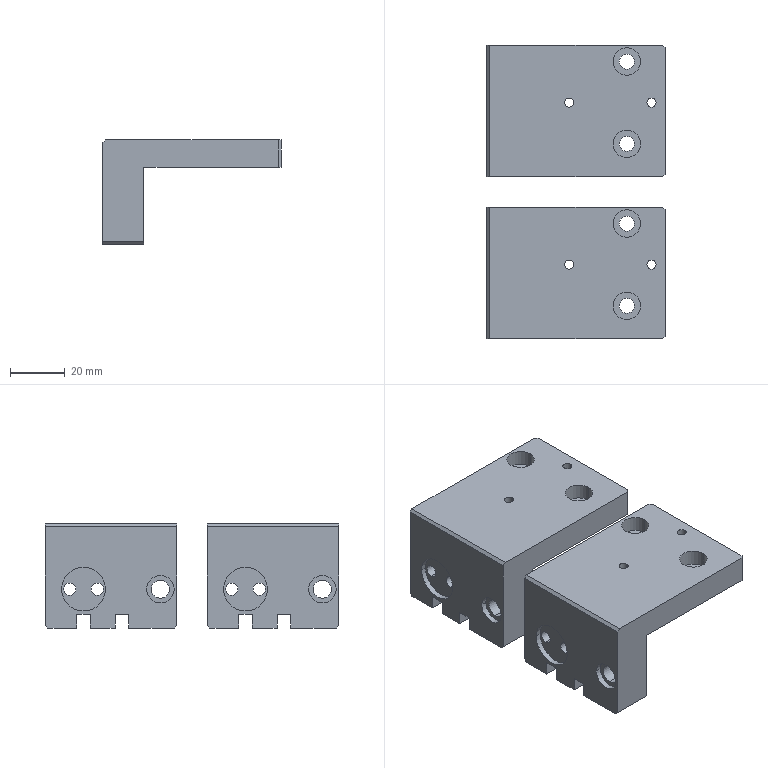NC program | NX | posted with a generic post | part box 65 x 107 x 38 mm
Lines 5400 to 5955 of 5955:
(ZLEVEL_PROFILE_COPY_1 , TOOL : D10JING)
N10774 T14 M6
N10776 G54
N10778 G17 G0 G90 X0.5 Y-6.567 B0. C0. S9500 M3
N10780 G43 Z30. H14
N10782 Z1.5
N10784 G94 G1 Y33.049 Z-0.576 F1000.
N10786 X0.828 Y34.364 Z-0.647
N10788 X1.496 Y35.545 Z-0.718
N10790 X2.455 Y36.504 Z-0.789
N10792 X3.636 Y37.172 Z-0.86
N10794 X4.951 Y37.5 Z-0.932
N10796 X54.049 Z-3.505
N10798 X55.364 Y37.172 Z-3.576
N10800 X56.545 Y36.504 Z-3.647
N10802 X57.504 Y35.545 Z-3.718
N10804 X58.172 Y34.364 Z-3.789
N10806 X58.5 Y33.049 Z-3.86
N10808 Y-32.049 Z-7.272
N10810 X58.147 Y-33.425 Z-7.346
N10812 X57.423 Y-34.648 Z-7.421
N10814 X55.648 Y-36.423 Z-7.552
N10816 X54.425 Y-37.147 Z-7.627
N10818 X53.049 Y-37.5 Z-7.701
N10820 X5.951 Z-10.169
N10822 X4.575 Y-37.147 Z-10.244
N10824 X3.352 Y-36.423 Z-10.318
N10826 X1.577 Y-34.648 Z-10.45
N10828 X0.853 Y-33.425 Z-10.524
N10830 X0.5 Y-32.049 Z-10.599
N10832 Y33.049 Z-14.01
N10834 X0.828 Y34.364 Z-14.081
N10836 X1.496 Y35.545 Z-14.153
N10838 X2.455 Y36.504 Z-14.224
N10840 X3.636 Y37.172 Z-14.295
N10842 X4.951 Y37.5 Z-14.366
N10844 X54.049 Z-16.939
N10846 X55.364 Y37.172 Z-17.01
N10848 X56.545 Y36.504 Z-17.081
N10850 X57.504 Y35.545 Z-17.152
N10852 X58.172 Y34.364 Z-17.223
N10854 X58.5 Y33.049 Z-17.294
N10856 Y0.5 Z-19.
N10858 Y-31.5 F1200.
N10860 G2 X57.036 Y-35.036 R5.
N10862 G1 X56.036 Y-36.036
N10864 G2 X52.5 Y-37.5 R5.
N10866 G1 X6.5
N10868 G2 X2.964 Y-36.036 R5.
N10870 G1 X1.964 Y-35.036
N10872 G2 X0.5 Y-31.5 R5.
N10874 G1 Y32.5
N10876 G2 X5.5 Y37.5 R5.
N10878 G1 X53.5
N10880 G2 X58.5 Y32.5 R5.
N10882 G1 Y0.5
N10884 Y-31.5 Z-21.373
N10886 X58.476 Y-31.99 Z-21.41
N10888 X58.404 Y-32.475 Z-21.446
N10890 X58.285 Y-32.951 Z-21.482
N10892 X58.119 Y-33.413 Z-21.519
N10894 X57.91 Y-33.857 Z-21.555
N10896 X57.657 Y-34.278 Z-21.591
N10898 X57.365 Y-34.672 Z-21.628
N10900 X57.036 Y-35.036 Z-21.664
N10902 X56.036 Y-36.036 Z-21.769
N10904 X55.672 Y-36.365 Z-21.805
N10906 X55.278 Y-36.657 Z-21.842
N10908 X54.857 Y-36.91 Z-21.878
N10910 X54.413 Y-37.119 Z-21.914
N10912 X53.951 Y-37.285 Z-21.951
N10914 X53.475 Y-37.404 Z-21.987
N10916 X52.99 Y-37.476 Z-22.023
N10918 X52.5 Y-37.5 Z-22.06
N10920 X6.5 Z-25.471
N10922 X6.01 Y-37.476 Z-25.507
N10924 X5.525 Y-37.404 Z-25.544
N10926 X5.049 Y-37.285 Z-25.58
N10928 X4.587 Y-37.119 Z-25.616
N10930 X4.143 Y-36.91 Z-25.653
N10932 X3.722 Y-36.657 Z-25.689
N10934 X3.328 Y-36.365 Z-25.726
N10936 X2.964 Y-36.036 Z-25.762
N10938 X1.964 Y-35.036 Z-25.867
N10940 X1.635 Y-34.672 Z-25.903
N10942 X1.343 Y-34.278 Z-25.939
N10944 X1.09 Y-33.857 Z-25.976
N10946 X0.881 Y-33.413 Z-26.012
N10948 X0.715 Y-32.951 Z-26.048
N10950 X0.596 Y-32.475 Z-26.085
N10952 X0.524 Y-31.99 Z-26.121
N10954 X0.5 Y-31.5 Z-26.158
N10956 Y32.5 Z-30.904
N10958 X0.524 Y32.99 Z-30.94
N10960 X0.596 Y33.475 Z-30.977
N10962 X0.715 Y33.951 Z-31.013
N10964 X0.881 Y34.413 Z-31.049
N10966 X1.09 Y34.857 Z-31.086
N10968 X1.343 Y35.278 Z-31.122
N10970 X1.635 Y35.672 Z-31.158
N10972 X1.964 Y36.036 Z-31.195
N10974 X2.328 Y36.365 Z-31.231
N10976 X2.722 Y36.657 Z-31.267
N10978 X3.143 Y36.91 Z-31.304
N10980 X3.587 Y37.119 Z-31.34
N10982 X4.049 Y37.285 Z-31.376
N10984 X4.525 Y37.404 Z-31.413
N10986 X5.01 Y37.476 Z-31.449
N10988 X5.5 Y37.5 Z-31.485
N10990 X53.5 Z-35.045
N10992 X53.99 Y37.476 Z-35.082
N10994 X54.475 Y37.404 Z-35.118
N10996 X54.951 Y37.285 Z-35.154
N10998 X55.413 Y37.119 Z-35.191
N11000 X55.857 Y36.91 Z-35.227
N11002 X56.278 Y36.657 Z-35.263
N11004 X56.672 Y36.365 Z-35.3
N11006 X57.036 Y36.036 Z-35.336
N11008 X57.365 Y35.672 Z-35.372
N11010 X57.657 Y35.278 Z-35.409
N11012 X57.91 Y34.857 Z-35.445
N11014 X58.119 Y34.413 Z-35.481
N11016 X58.285 Y33.951 Z-35.518
N11018 X58.404 Y33.475 Z-35.554
N11020 X58.476 Y32.99 Z-35.59
N11022 X58.5 Y32.5 Z-35.627
N11024 Y0.5 Z-38.
N11026 Y-31.5
N11028 G2 X57.036 Y-35.036 R5.
N11030 G1 X56.036 Y-36.036
N11032 G2 X52.5 Y-37.5 R5.
N11034 G1 X6.5
N11036 G2 X2.964 Y-36.036 R5.
N11038 G1 X1.964 Y-35.036
N11040 G2 X0.5 Y-31.5 R5.
N11042 G1 Y32.5
N11044 G2 X5.5 Y37.5 R5.
N11046 G1 X53.5
N11048 G2 X58.5 Y32.5 R5.
N11050 G1 Y0.5
N11052 Z-36.5
N11054 G0 Z53.
N11056 X-0.5 Y6.739
N11058 Z1.5
N11060 G1 Y-32.049 Z-0.533 F1000.
N11062 X-0.853 Y-33.425 Z-0.607
N11064 X-1.577 Y-34.648 Z-0.682
N11066 X-3.352 Y-36.423 Z-0.813
N11068 X-4.575 Y-37.147 Z-0.888
N11070 X-5.951 Y-37.5 Z-0.962
N11072 X-53.049 Z-3.431
N11074 X-54.425 Y-37.147 Z-3.505
N11076 X-55.648 Y-36.423 Z-3.579
N11078 X-57.423 Y-34.648 Z-3.711
N11080 X-58.147 Y-33.425 Z-3.786
N11082 X-58.5 Y-32.049 Z-3.86
N11084 Y33.049 Z-7.272
N11086 X-58.172 Y34.364 Z-7.343
N11088 X-57.504 Y35.545 Z-7.414
N11090 X-56.545 Y36.504 Z-7.485
N11092 X-55.364 Y37.172 Z-7.556
N11094 X-54.049 Y37.5 Z-7.627
N11096 X-4.951 Z-10.2
N11098 X-3.636 Y37.172 Z-10.271
N11100 X-2.455 Y36.504 Z-10.342
N11102 X-1.496 Y35.545 Z-10.413
N11104 X-0.828 Y34.364 Z-10.484
N11106 X-0.5 Y33.049 Z-10.555
N11108 Y-32.049 Z-13.967
N11110 X-0.853 Y-33.425 Z-14.041
N11112 X-1.577 Y-34.648 Z-14.116
N11114 X-3.352 Y-36.423 Z-14.248
N11116 X-4.575 Y-37.147 Z-14.322
N11118 X-5.951 Y-37.5 Z-14.396
N11120 X-53.049 Z-16.865
N11122 X-54.425 Y-37.147 Z-16.939
N11124 X-55.648 Y-36.423 Z-17.014
N11126 X-57.423 Y-34.648 Z-17.145
N11128 X-58.147 Y-33.425 Z-17.22
N11130 X-58.5 Y-32.049 Z-17.294
N11132 Y0.5 Z-19.
N11134 Y32.5 F1200.
N11136 G2 X-53.5 Y37.5 R5.
N11138 G1 X-5.5
N11140 G2 X-0.5 Y32.5 R5.
N11142 G1 Y-31.5
N11144 G2 X-1.964 Y-35.036 R5.
N11146 G1 X-2.964 Y-36.036
N11148 G2 X-6.5 Y-37.5 R5.
N11150 G1 X-52.5
N11152 G2 X-56.036 Y-36.036 R5.
N11154 G1 X-57.036 Y-35.036
N11156 G2 X-58.5 Y-31.5 R5.
N11158 G1 Y0.5
N11160 Y32.5 Z-21.373
N11162 X-58.476 Y32.99 Z-21.41
N11164 X-58.404 Y33.475 Z-21.446
N11166 X-58.285 Y33.951 Z-21.482
N11168 X-58.119 Y34.413 Z-21.519
N11170 X-57.91 Y34.857 Z-21.555
N11172 X-57.657 Y35.278 Z-21.591
N11174 X-57.365 Y35.672 Z-21.628
N11176 X-57.036 Y36.036 Z-21.664
N11178 X-56.672 Y36.365 Z-21.7
N11180 X-56.278 Y36.657 Z-21.737
N11182 X-55.857 Y36.91 Z-21.773
N11184 X-55.413 Y37.119 Z-21.809
N11186 X-54.951 Y37.285 Z-21.846
N11188 X-54.475 Y37.404 Z-21.882
N11190 X-53.99 Y37.476 Z-21.918
N11192 X-53.5 Y37.5 Z-21.955
N11194 X-5.5 Z-25.515
N11196 X-5.01 Y37.476 Z-25.551
N11198 X-4.525 Y37.404 Z-25.587
N11200 X-4.049 Y37.285 Z-25.624
N11202 X-3.587 Y37.119 Z-25.66
N11204 X-3.143 Y36.91 Z-25.696
N11206 X-2.722 Y36.657 Z-25.733
N11208 X-2.328 Y36.365 Z-25.769
N11210 X-1.964 Y36.036 Z-25.805
N11212 X-1.635 Y35.672 Z-25.842
N11214 X-1.343 Y35.278 Z-25.878
N11216 X-1.09 Y34.857 Z-25.914
N11218 X-0.881 Y34.413 Z-25.951
N11220 X-0.715 Y33.951 Z-25.987
N11222 X-0.596 Y33.475 Z-26.023
N11224 X-0.524 Y32.99 Z-26.06
N11226 X-0.5 Y32.5 Z-26.096
N11228 Y-31.5 Z-30.842
N11230 X-0.524 Y-31.99 Z-30.879
N11232 X-0.596 Y-32.475 Z-30.915
N11234 X-0.715 Y-32.951 Z-30.952
N11236 X-0.881 Y-33.413 Z-30.988
N11238 X-1.09 Y-33.857 Z-31.024
N11240 X-1.343 Y-34.278 Z-31.061
N11242 X-1.635 Y-34.672 Z-31.097
N11244 X-1.964 Y-35.036 Z-31.133
N11246 X-2.964 Y-36.036 Z-31.238
N11248 X-3.328 Y-36.365 Z-31.274
N11250 X-3.722 Y-36.657 Z-31.311
N11252 X-4.143 Y-36.91 Z-31.347
N11254 X-4.587 Y-37.119 Z-31.384
N11256 X-5.049 Y-37.285 Z-31.42
N11258 X-5.525 Y-37.404 Z-31.456
N11260 X-6.01 Y-37.476 Z-31.493
N11262 X-6.5 Y-37.5 Z-31.529
N11264 X-52.5 Z-34.94
N11266 X-52.99 Y-37.476 Z-34.977
N11268 X-53.475 Y-37.404 Z-35.013
N11270 X-53.951 Y-37.285 Z-35.049
N11272 X-54.413 Y-37.119 Z-35.086
N11274 X-54.857 Y-36.91 Z-35.122
N11276 X-55.278 Y-36.657 Z-35.158
N11278 X-55.672 Y-36.365 Z-35.195
N11280 X-56.036 Y-36.036 Z-35.231
N11282 X-57.036 Y-35.036 Z-35.336
N11284 X-57.365 Y-34.672 Z-35.372
N11286 X-57.657 Y-34.278 Z-35.409
N11288 X-57.91 Y-33.857 Z-35.445
N11290 X-58.119 Y-33.413 Z-35.481
N11292 X-58.285 Y-32.951 Z-35.518
N11294 X-58.404 Y-32.475 Z-35.554
N11296 X-58.476 Y-31.99 Z-35.59
N11298 X-58.5 Y-31.5 Z-35.627
N11300 Y0.5 Z-38.
N11302 Y32.5
N11304 G2 X-53.5 Y37.5 R5.
N11306 G1 X-5.5
N11308 G2 X-0.5 Y32.5 R5.
N11310 G1 Y-31.5
N11312 G2 X-1.964 Y-35.036 R5.
N11314 G1 X-2.964 Y-36.036
N11316 G2 X-6.5 Y-37.5 R5.
N11318 G1 X-52.5
N11320 G2 X-56.036 Y-36.036 R5.
N11322 G1 X-57.036 Y-35.036
N11324 G2 X-58.5 Y-31.5 R5.
N11326 G1 Y0.5
N11328 Z-36.5
N11330 G0 Z30.
N11332 M5
(HOLE_MILLING , TOOL : D6)
N11334 T12 M6
N11336 G54
N11338 G17 G0 G90 X-41.5 Y-18.5 B0. C0. S9500 M3
N11340 G43 Z30. H12
N11342 Z0.5
N11344 G94 G3 X-42.5 Y-19.5 R1. F1500.
N11346 X-41.5 Y-20.5 R1.
N11348 X-41.5 Y-20.5 Z0. I0. J2.
N11350 X-41.5 Y-20.5 Z-0.5 I0. J2.
N11352 X-41.5 Y-20.5 Z-1. I0. J2.
N11354 X-41.5 Y-20.5 Z-1.5 I0. J2.
N11356 X-41.5 Y-20.5 Z-2. I0. J2.
N11358 X-41.5 Y-20.5 Z-2.5 I0. J2.
N11360 X-41.5 Y-20.5 Z-3. I0. J2.
N11362 X-41.5 Y-20.5 Z-3.5 I0. J2.
N11364 X-41.5 Y-20.5 Z-4. I0. J2.
N11366 X-41.5 Y-20.5 Z-4.5 I0. J2.
N11368 X-41.5 Y-20.5 Z-5. I0. J2.
N11370 X-41.5 Y-20.5 Z-5.5 I0. J2.
N11372 X-40.324 Y-16.882 Z-5.7 R2.
N11374 X-43.118 Y-17.324 R2.
N11376 X-40.324 Y-16.882 R-2.
N11378 X-41.721 Y-17.103 R1.
N11380 X-41.5 Y-18.5 R1.
N11382 G0 Z30.
N11384 X-11.5
N11386 Z0.5
N11388 G3 X-12.5 Y-19.5 R1.
N11390 X-11.5 Y-20.5 R1.
N11392 X-11.5 Y-20.5 Z0. I0. J2.
N11394 X-11.5 Y-20.5 Z-0.5 I0. J2.
N11396 X-11.5 Y-20.5 Z-1. I0. J2.
N11398 X-11.5 Y-20.5 Z-1.5 I0. J2.
N11400 X-11.5 Y-20.5 Z-2. I0. J2.
N11402 X-11.5 Y-20.5 Z-2.5 I0. J2.
N11404 X-11.5 Y-20.5 Z-3. I0. J2.
N11406 X-11.5 Y-20.5 Z-3.5 I0. J2.
N11408 X-11.5 Y-20.5 Z-4. I0. J2.
N11410 X-11.5 Y-20.5 Z-4.5 I0. J2.
N11412 X-11.5 Y-20.5 Z-5. I0. J2.
N11414 X-11.5 Y-20.5 Z-5.5 I0. J2.
N11416 X-10.324 Y-16.882 Z-5.7 R2.
N11418 X-13.118 Y-17.324 R2.
N11420 X-10.324 Y-16.882 R-2.
N11422 X-11.721 Y-17.103 R1.
N11424 X-11.5 Y-18.5 R1.
N11426 G0 Z30.
N11428 X17.5
N11430 Z0.5
N11432 G3 X16.5 Y-19.5 R1.
N11434 X17.5 Y-20.5 R1.
N11436 X17.5 Y-20.5 Z0. I0. J2.
N11438 X17.5 Y-20.5 Z-0.5 I0. J2.
N11440 X17.5 Y-20.5 Z-1. I0. J2.
N11442 X17.5 Y-20.5 Z-1.5 I0. J2.
N11444 X17.5 Y-20.5 Z-2. I0. J2.
N11446 X17.5 Y-20.5 Z-2.5 I0. J2.
N11448 X17.5 Y-20.5 Z-3. I0. J2.
N11450 X17.5 Y-20.5 Z-3.5 I0. J2.
N11452 X17.5 Y-20.5 Z-4. I0. J2.
N11454 X17.5 Y-20.5 Z-4.5 I0. J2.
N11456 X17.5 Y-20.5 Z-5. I0. J2.
N11458 X17.5 Y-20.5 Z-5.5 I0. J2.
N11460 X18.676 Y-16.882 Z-5.7 R2.
N11462 X15.882 Y-17.324 R2.
N11464 X18.676 Y-16.882 R-2.
N11466 X17.279 Y-17.103 R1.
N11468 X17.5 Y-18.5 R1.
N11470 G0 Z30.
N11472 X47.5
N11474 Z0.5
N11476 G3 X46.5 Y-19.5 R1.
N11478 X47.5 Y-20.5 R1.
N11480 X47.5 Y-20.5 Z0. I0. J2.
N11482 X47.5 Y-20.5 Z-0.5 I0. J2.
N11484 X47.5 Y-20.5 Z-1. I0. J2.
N11486 X47.5 Y-20.5 Z-1.5 I0. J2.
N11488 X47.5 Y-20.5 Z-2. I0. J2.
N11490 X47.5 Y-20.5 Z-2.5 I0. J2.
N11492 X47.5 Y-20.5 Z-3. I0. J2.
N11494 X47.5 Y-20.5 Z-3.5 I0. J2.
N11496 X47.5 Y-20.5 Z-4. I0. J2.
N11498 X47.5 Y-20.5 Z-4.5 I0. J2.
N11500 X47.5 Y-20.5 Z-5. I0. J2.
N11502 X47.5 Y-20.5 Z-5.5 I0. J2.
N11504 X48.676 Y-16.882 Z-5.7 R2.
N11506 X45.882 Y-17.324 R2.
N11508 X48.676 Y-16.882 R-2.
N11510 X47.279 Y-17.103 R1.
N11512 X47.5 Y-18.5 R1.
N11514 G0 Z30.
N11516 M5
(PLANAR_MILL_COPY_COPY_COPY , TOOL : D6A45)
N11518 T01 M6
N11520 G54
N11522 G17 G0 G90 X-27. Y2.933 B0. C0. S9500 M3
N11524 G43 Z30. H1
N11526 Z0.5
N11528 G94 G1 Z-1. F1250.
N11530 G3 X-27.25 Y2.5 R0.5
N11532 X-26.5 Y1.75 R0.75
N11534 X-27.25 Y2.5 R-0.75
N11536 X-27. Y2.067 R0.5
N11538 G1 Z0.5
N11540 G0 Z30.
N11542 X-54.9 Y-0.366
N11544 Z0.5
N11546 G1 Z-1.
N11548 G3 X-54.4 Y0.5 R1.
N11550 G1 Y32.5
N11552 G2 X-53.5 Y33.4 R0.9
N11554 G1 X-5.5
N11556 G2 X-4.6 Y32.5 R0.9
N11558 G1 Y-31.5
N11560 G2 X-4.864 Y-32.136 R0.9
N11562 G1 X-5.864 Y-33.136
N11564 G2 X-6.5 Y-33.4 R0.9
N11566 G1 X-52.5
N11568 G2 X-53.136 Y-33.136 R0.9
N11570 G1 X-54.136 Y-32.136
N11572 G2 X-54.4 Y-31.5 R0.9
N11574 G1 Y0.5
N11576 G3 X-54.9 Y1.366 R1.
N11578 G1 Z0.5
N11580 G0 Z30.
N11582 X-45.1 Y-17.634
N11584 Z0.5
N11586 G1 Z-1.
N11588 G3 X-45.6 Y-18.5 R1.
N11590 X-41.5 Y-22.6 R4.1
N11592 X-45.6 Y-18.5 R-4.1
N11594 X-45.1 Y-19.366 R1.
N11596 G1 Z0.5
N11598 G0 Z30.
N11600 X-26.933 Y-28.
N11602 Z0.5
N11604 G1 Z-1.
N11606 G3 X-26.5 Y-28.25 R0.5
N11608 X-25.75 Y-27.5 R0.75
N11610 X-26.5 Y-28.25 R-0.75
N11612 X-26.067 Y-28. R0.5
N11614 G1 Z0.5
N11616 G0 Z30.
N11618 X-12.366 Y-22.1
N11620 Z0.5
N11622 G1 Z-1.
N11624 G3 X-11.5 Y-22.6 R1.
N11626 X-7.4 Y-18.5 R4.1
N11628 X-11.5 Y-22.6 R-4.1
N11630 X-10.634 Y-22.1 R1.
N11632 G1 Z0.5
N11634 G0 Z30.
N11636 X16.634
N11638 Z0.5
N11640 G1 Z-1.
N11642 G3 X17.5 Y-22.6 R1.
N11644 X21.6 Y-18.5 R4.1
N11646 X17.5 Y-22.6 R-4.1
N11648 X18.366 Y-22.1 R1.
N11650 G1 Z0.5
N11652 G0 Z30.
N11654 X32.067 Y-28.
N11656 Z0.5
N11658 G1 Z-1.
N11660 G3 X32.5 Y-28.25 R0.5
N11662 X33.25 Y-27.5 R0.75
N11664 X32.5 Y-28.25 R-0.75
N11666 X32.933 Y-28. R0.5
N11668 G1 Z0.5
N11670 G0 Z30.
N11672 X51.1 Y-19.366
N11674 Z0.5
N11676 G1 Z-1.
N11678 G3 X51.6 Y-18.5 R1.
N11680 X47.5 Y-14.4 R4.1
N11682 X51.6 Y-18.5 R-4.1
N11684 X51.1 Y-17.634 R1.
N11686 G1 Z0.5
N11688 G0 Z30.
N11690 X33. Y2.067
N11692 Z0.5
N11694 G1 Z-1.
N11696 G3 X33.25 Y2.5 R0.5
N11698 X32.5 Y3.25 R0.75
N11700 X33.25 Y2.5 R-0.75
N11702 X33. Y2.933 R0.5
N11704 G1 Z0.5
N11706 G0 Z30.
N11708 X54.9 Y1.366
N11710 Z0.5
N11712 G1 Z-1.
N11714 G3 X54.4 Y0.5 R1.
N11716 G1 Y-31.5
N11718 G2 X54.136 Y-32.136 R0.9
N11720 G1 X53.136 Y-33.136
N11722 G2 X52.5 Y-33.4 R0.9
N11724 G1 X6.5
N11726 G2 X5.864 Y-33.136 R0.9
N11728 G1 X4.864 Y-32.136
N11730 G2 X4.6 Y-31.5 R0.9
N11732 G1 Y32.5
N11734 G2 X5.5 Y33.4 R0.9
N11736 G1 X53.5
N11738 G2 X54.4 Y32.5 R0.9
N11740 G1 Y0.5
N11742 G3 X54.9 Y-0.366 R1.
N11744 G1 Z0.5
N11746 G0 Z30.
(PLANAR_MILL_COPY_COPY_COPY_COPY_1 , TOOL : D6A45)
N11748 X-54.366 Y33.5
N11750 Z0.
N11752 G1 Z-1.5
N11754 G3 X-53.5 Y33. R1.
N11756 G1 X-5.5
N11758 G3 X-4.634 Y33.5 R1.
N11760 G1 Z0.
N11762 G0 Z30.
N11764 X4.634
N11766 Z0.
N11768 G1 Z-1.5
N11770 G3 X5.5 Y33. R1.
N11772 G1 X53.5
N11774 G3 X54.366 Y33.5 R1.
N11776 G1 Z0.
N11778 G0 Z30.
(PLANAR_MILL_COPY_COPY_COPY_COPY_1_COPY , TOOL : D6A45)
N11780 X-27.1 Y2.933
N11782 Z0.
N11784 G1 Z-1.5
N11786 G3 X-27.35 Y2.5 R0.5
N11788 X-26.5 Y1.65 R0.85
N11790 X-27.35 Y2.5 R-0.85
N11792 X-27.1 Y2.067 R0.5
N11794 G1 Z0.
N11796 G0 Z30.
N11798 Y-27.067
N11800 Z0.
N11802 G1 Z-1.5
N11804 G3 X-27.35 Y-27.5 R0.5
N11806 X-26.5 Y-28.35 R0.85
N11808 X-27.35 Y-27.5 R-0.85
N11810 X-27.1 Y-27.933 R0.5
N11812 G1 Z0.
N11814 G0 Z30.
N11816 X33.1
N11818 Z0.
N11820 G1 Z-1.5
N11822 G3 X33.35 Y-27.5 R0.5
N11824 X32.5 Y-26.65 R0.85
N11826 X33.35 Y-27.5 R-0.85
N11828 X33.1 Y-27.067 R0.5
N11830 G1 Z0.
N11832 G0 Z30.
N11834 X32.933 Y3.1
N11836 Z0.
N11838 G1 Z-1.5
N11840 G3 X32.5 Y3.35 R0.5
N11842 X31.65 Y2.5 R0.85
N11844 X32.5 Y3.35 R-0.85
N11846 X32.067 Y3.1 R0.5
N11848 G1 Z0.
N11850 G0 Z30.
N11852 M5
N11854 M2